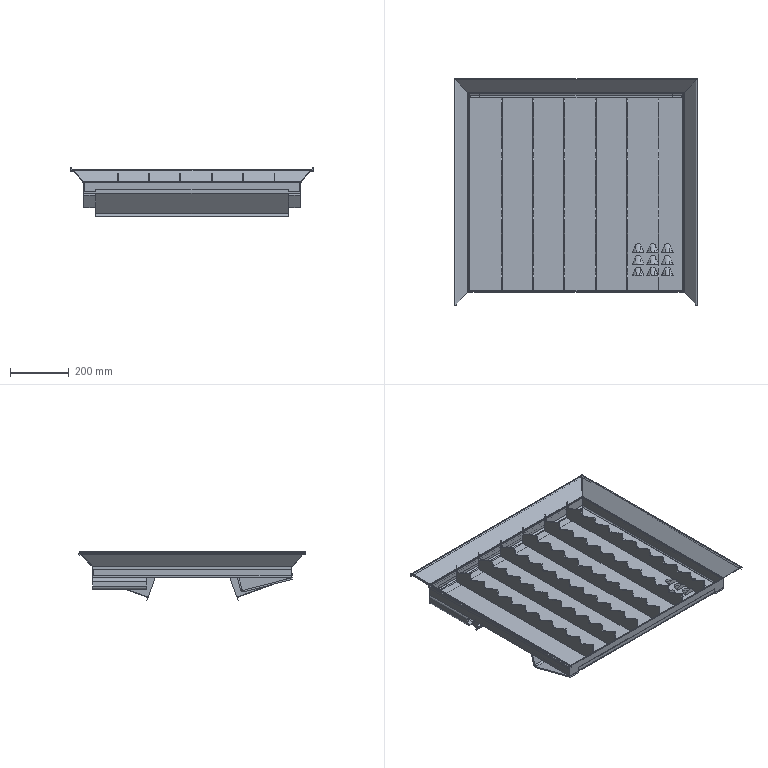Part | SolidWorks | features LayoutProfileFeature 1 | 20 solids | 446 faces | box 829.179 x 774.462 x 164.679 mm | volume 3231885 mm3 | plane 333 | cylinder 80 | spline 33 | commonest cylinder face diameters 2 x16 14 x16 4 x11 16 x8 24 x8 10 x6